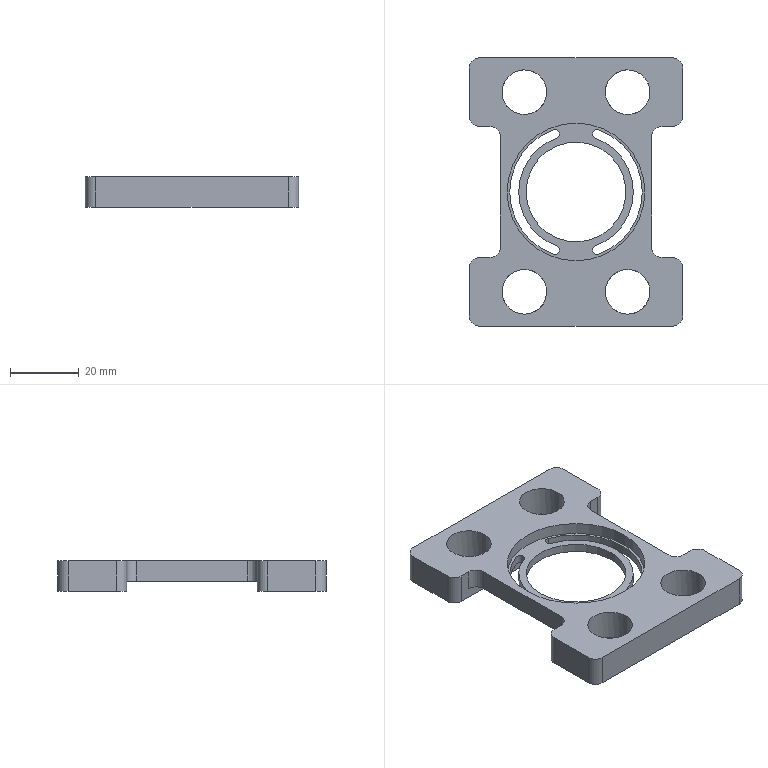Part | 1 solid | 41 faces | box 62 x 78 x 9 mm | volume 20835 mm3 | cylinder 26 | plane 15 | commonest cylinder face diameters 6 x12 2.6 x4 13 x4 33.3 x2 38.5 x2 29 x1
STEP:
#1=CARTESIAN_POINT('',(-25.,-19.,-6.));
#2=VERTEX_POINT('',#1);
#3=CARTESIAN_POINT('',(25.,-19.,-6.));
#4=VERTEX_POINT('',#3);
#5=CARTESIAN_POINT('',(28.,-19.,-6.));
#6=DIRECTION('',(1.,0.,0.));
#7=VECTOR('',#6,1000.);
#8=LINE('',#5,#7);
#9=EDGE_CURVE('',#2,#4,#8,.T.);
#10=ORIENTED_EDGE('',*,*,#9,.F.);
#11=CARTESIAN_POINT('',(-22.,-16.,-6.));
#12=VERTEX_POINT('',#11);
#13=CARTESIAN_POINT('',(-25.,-16.,-6.));
#14=DIRECTION('',(0.,0.,1.));
#15=DIRECTION('',(-1.,0.,0.));
#16=AXIS2_PLACEMENT_3D('',#13,#14,#15);
#17=CIRCLE('',#16,3.);
#18=EDGE_CURVE('',#2,#12,#17,.T.);
#19=ORIENTED_EDGE('',*,*,#18,.T.);
#20=CARTESIAN_POINT('',(-22.,16.,-6.));
#21=VERTEX_POINT('',#20);
#22=CARTESIAN_POINT('',(-22.,-35.,-6.));
#23=DIRECTION('',(0.,1.,0.));
#24=VECTOR('',#23,1000.);
#25=LINE('',#22,#24);
#26=EDGE_CURVE('',#12,#21,#25,.T.);
#27=ORIENTED_EDGE('',*,*,#26,.T.);
#28=CARTESIAN_POINT('',(-25.,19.,-6.));
#29=VERTEX_POINT('',#28);
#30=CARTESIAN_POINT('',(-25.,16.,-6.));
#31=DIRECTION('',(0.,0.,1.));
#32=DIRECTION('',(-1.,0.,0.));
#33=AXIS2_PLACEMENT_3D('',#30,#31,#32);
#34=CIRCLE('',#33,3.);
#35=EDGE_CURVE('',#21,#29,#34,.T.);
#36=ORIENTED_EDGE('',*,*,#35,.T.);
#37=CARTESIAN_POINT('',(25.,19.,-6.));
#38=VERTEX_POINT('',#37);
#39=CARTESIAN_POINT('',(-28.,19.,-6.));
#40=DIRECTION('',(-1.,0.,0.));
#41=VECTOR('',#40,1000.);
#42=LINE('',#39,#41);
#43=EDGE_CURVE('',#38,#29,#42,.T.);
#44=ORIENTED_EDGE('',*,*,#43,.F.);
#45=CARTESIAN_POINT('',(22.,16.,-6.));
#46=VERTEX_POINT('',#45);
#47=CARTESIAN_POINT('',(25.,16.,-6.));
#48=DIRECTION('',(0.,0.,1.));
#49=DIRECTION('',(-1.,0.,0.));
#50=AXIS2_PLACEMENT_3D('',#47,#48,#49);
#51=CIRCLE('',#50,3.);
#52=EDGE_CURVE('',#38,#46,#51,.T.);
#53=ORIENTED_EDGE('',*,*,#52,.T.);
#54=CARTESIAN_POINT('',(22.,-16.,-6.));
#55=VERTEX_POINT('',#54);
#56=CARTESIAN_POINT('',(22.,35.,-6.));
#57=DIRECTION('',(0.,-1.,0.));
#58=VECTOR('',#57,1000.);
#59=LINE('',#56,#58);
#60=EDGE_CURVE('',#46,#55,#59,.T.);
#61=ORIENTED_EDGE('',*,*,#60,.T.);
#62=CARTESIAN_POINT('',(25.,-16.,-6.));
#63=DIRECTION('',(0.,0.,1.));
#64=DIRECTION('',(-1.,0.,0.));
#65=AXIS2_PLACEMENT_3D('',#62,#63,#64);
#66=CIRCLE('',#65,3.);
#67=EDGE_CURVE('',#55,#4,#66,.T.);
#68=ORIENTED_EDGE('',*,*,#67,.T.);
#69=EDGE_LOOP('',(#10,#19,#27,#36,#44,#53,#61,#68));
#70=FACE_BOUND('',#69,.T.);
#71=CARTESIAN_POINT('',(-5.695,-15.646,-6.));
#72=VERTEX_POINT('',#71);
#73=CARTESIAN_POINT('',(-5.695,15.646,-6.));
#74=VERTEX_POINT('',#73);
#75=CARTESIAN_POINT('',(0.,0.,-6.));
#76=DIRECTION('',(0.,0.,-1.));
#77=DIRECTION('',(0.,1.,0.));
#78=AXIS2_PLACEMENT_3D('',#75,#76,#77);
#79=CIRCLE('',#78,16.65);
#80=EDGE_CURVE('',#72,#74,#79,.T.);
#81=ORIENTED_EDGE('',*,*,#80,.T.);
#82=CARTESIAN_POINT('',(-6.584,18.089,-6.));
#83=VERTEX_POINT('',#82);
#84=CARTESIAN_POINT('',(-6.139,16.867,-6.));
#85=DIRECTION('',(0.,0.,1.));
#86=DIRECTION('',(0.,-1.,0.));
#87=AXIS2_PLACEMENT_3D('',#84,#85,#86);
#88=CIRCLE('',#87,1.3);
#89=EDGE_CURVE('',#74,#83,#88,.T.);
#90=ORIENTED_EDGE('',*,*,#89,.T.);
#91=CARTESIAN_POINT('',(-6.584,-18.089,-6.));
#92=VERTEX_POINT('',#91);
#93=CARTESIAN_POINT('',(0.,0.,-6.));
#94=DIRECTION('',(0.,0.,1.));
#95=DIRECTION('',(0.,1.,0.));
#96=AXIS2_PLACEMENT_3D('',#93,#94,#95);
#97=CIRCLE('',#96,19.25);
#98=EDGE_CURVE('',#83,#92,#97,.T.);
#99=ORIENTED_EDGE('',*,*,#98,.T.);
#100=CARTESIAN_POINT('',(-6.139,-16.867,-6.));
#101=DIRECTION('',(0.,0.,1.));
#102=DIRECTION('',(0.,1.,0.));
#103=AXIS2_PLACEMENT_3D('',#100,#101,#102);
#104=CIRCLE('',#103,1.3);
#105=EDGE_CURVE('',#92,#72,#104,.T.);
#106=ORIENTED_EDGE('',*,*,#105,.T.);
#107=EDGE_LOOP('',(#81,#90,#99,#106));
#108=FACE_BOUND('',#107,.T.);
#109=CARTESIAN_POINT('',(6.584,18.089,-6.));
#110=VERTEX_POINT('',#109);
#111=CARTESIAN_POINT('',(5.695,15.646,-6.));
#112=VERTEX_POINT('',#111);
#113=CARTESIAN_POINT('',(6.139,16.867,-6.));
#114=DIRECTION('',(0.,0.,1.));
#115=DIRECTION('',(0.,-1.,0.));
#116=AXIS2_PLACEMENT_3D('',#113,#114,#115);
#117=CIRCLE('',#116,1.3);
#118=EDGE_CURVE('',#110,#112,#117,.T.);
#119=ORIENTED_EDGE('',*,*,#118,.T.);
#120=CARTESIAN_POINT('',(5.695,-15.646,-6.));
#121=VERTEX_POINT('',#120);
#122=CARTESIAN_POINT('',(0.,0.,-6.));
#123=DIRECTION('',(0.,0.,-1.));
#124=DIRECTION('',(0.,1.,0.));
#125=AXIS2_PLACEMENT_3D('',#122,#123,#124);
#126=CIRCLE('',#125,16.65);
#127=EDGE_CURVE('',#112,#121,#126,.T.);
#128=ORIENTED_EDGE('',*,*,#127,.T.);
#129=CARTESIAN_POINT('',(6.584,-18.089,-6.));
#130=VERTEX_POINT('',#129);
#131=CARTESIAN_POINT('',(6.139,-16.867,-6.));
#132=DIRECTION('',(0.,0.,1.));
#133=DIRECTION('',(0.,1.,0.));
#134=AXIS2_PLACEMENT_3D('',#131,#132,#133);
#135=CIRCLE('',#134,1.3);
#136=EDGE_CURVE('',#121,#130,#135,.T.);
#137=ORIENTED_EDGE('',*,*,#136,.T.);
#138=CARTESIAN_POINT('',(0.,0.,-6.));
#139=DIRECTION('',(0.,0.,1.));
#140=DIRECTION('',(0.,1.,0.));
#141=AXIS2_PLACEMENT_3D('',#138,#139,#140);
#142=CIRCLE('',#141,19.25);
#143=EDGE_CURVE('',#130,#110,#142,.T.);
#144=ORIENTED_EDGE('',*,*,#143,.T.);
#145=EDGE_LOOP('',(#119,#128,#137,#144));
#146=FACE_BOUND('',#145,.T.);
#147=CARTESIAN_POINT('',(-14.5,0.,-6.));
#148=VERTEX_POINT('',#147);
#149=CARTESIAN_POINT('',(0.,0.,-6.));
#150=DIRECTION('',(0.,0.,1.));
#151=DIRECTION('',(-1.,0.,0.));
#152=AXIS2_PLACEMENT_3D('',#149,#150,#151);
#153=CIRCLE('',#152,14.5);
#154=EDGE_CURVE('',#148,#148,#153,.T.);
#155=ORIENTED_EDGE('',*,*,#154,.T.);
#156=EDGE_LOOP('',(#155));
#157=FACE_BOUND('',#156,.T.);
#158=CARTESIAN_POINT('',(0.,0.,-6.));
#159=DIRECTION('',(0.,0.,-1.));
#160=DIRECTION('',(1.,0.,0.));
#161=AXIS2_PLACEMENT_3D('',#158,#159,#160);
#162=PLANE('',#161);
#163=ADVANCED_FACE('',(#70,#108,#146,#157),#162,.T.);
#164=CARTESIAN_POINT('',(-5.695,15.646,-3.5));
#165=VERTEX_POINT('',#164);
#166=CARTESIAN_POINT('',(-6.584,18.089,-3.5));
#167=VERTEX_POINT('',#166);
#168=CARTESIAN_POINT('',(-6.139,16.867,-3.5));
#169=DIRECTION('',(0.,0.,1.));
#170=DIRECTION('',(-1.,0.,0.));
#171=AXIS2_PLACEMENT_3D('',#168,#169,#170);
#172=CIRCLE('',#171,1.3);
#173=EDGE_CURVE('',#165,#167,#172,.T.);
#174=ORIENTED_EDGE('',*,*,#173,.F.);
#175=CARTESIAN_POINT('',(-5.695,-15.646,-3.5));
#176=VERTEX_POINT('',#175);
#177=CARTESIAN_POINT('',(0.,0.,-3.5));
#178=DIRECTION('',(0.,0.,-1.));
#179=DIRECTION('',(-1.,0.,0.));
#180=AXIS2_PLACEMENT_3D('',#177,#178,#179);
#181=CIRCLE('',#180,16.65);
#182=EDGE_CURVE('',#176,#165,#181,.T.);
#183=ORIENTED_EDGE('',*,*,#182,.F.);
#184=CARTESIAN_POINT('',(-6.584,-18.089,-3.5));
#185=VERTEX_POINT('',#184);
#186=CARTESIAN_POINT('',(-6.139,-16.867,-3.5));
#187=DIRECTION('',(0.,0.,1.));
#188=DIRECTION('',(-1.,0.,0.));
#189=AXIS2_PLACEMENT_3D('',#186,#187,#188);
#190=CIRCLE('',#189,1.3);
#191=EDGE_CURVE('',#185,#176,#190,.T.);
#192=ORIENTED_EDGE('',*,*,#191,.F.);
#193=CARTESIAN_POINT('',(0.,0.,-3.5));
#194=DIRECTION('',(0.,0.,1.));
#195=DIRECTION('',(-1.,0.,0.));
#196=AXIS2_PLACEMENT_3D('',#193,#194,#195);
#197=CIRCLE('',#196,19.25);
#198=EDGE_CURVE('',#167,#185,#197,.T.);
#199=ORIENTED_EDGE('',*,*,#198,.F.);
#200=EDGE_LOOP('',(#174,#183,#192,#199));
#201=FACE_BOUND('',#200,.T.);
#202=CARTESIAN_POINT('',(5.695,15.646,-3.5));
#203=VERTEX_POINT('',#202);
#204=CARTESIAN_POINT('',(5.695,-15.646,-3.5));
#205=VERTEX_POINT('',#204);
#206=CARTESIAN_POINT('',(0.,0.,-3.5));
#207=DIRECTION('',(0.,0.,-1.));
#208=DIRECTION('',(-1.,0.,0.));
#209=AXIS2_PLACEMENT_3D('',#206,#207,#208);
#210=CIRCLE('',#209,16.65);
#211=EDGE_CURVE('',#203,#205,#210,.T.);
#212=ORIENTED_EDGE('',*,*,#211,.F.);
#213=CARTESIAN_POINT('',(6.584,18.089,-3.5));
#214=VERTEX_POINT('',#213);
#215=CARTESIAN_POINT('',(6.139,16.867,-3.5));
#216=DIRECTION('',(0.,0.,1.));
#217=DIRECTION('',(-1.,0.,0.));
#218=AXIS2_PLACEMENT_3D('',#215,#216,#217);
#219=CIRCLE('',#218,1.3);
#220=EDGE_CURVE('',#214,#203,#219,.T.);
#221=ORIENTED_EDGE('',*,*,#220,.F.);
#222=CARTESIAN_POINT('',(6.584,-18.089,-3.5));
#223=VERTEX_POINT('',#222);
#224=CARTESIAN_POINT('',(0.,0.,-3.5));
#225=DIRECTION('',(0.,0.,1.));
#226=DIRECTION('',(-1.,0.,0.));
#227=AXIS2_PLACEMENT_3D('',#224,#225,#226);
#228=CIRCLE('',#227,19.25);
#229=EDGE_CURVE('',#223,#214,#228,.T.);
#230=ORIENTED_EDGE('',*,*,#229,.F.);
#231=CARTESIAN_POINT('',(6.139,-16.867,-3.5));
#232=DIRECTION('',(0.,0.,1.));
#233=DIRECTION('',(-1.,0.,0.));
#234=AXIS2_PLACEMENT_3D('',#231,#232,#233);
#235=CIRCLE('',#234,1.3);
#236=EDGE_CURVE('',#205,#223,#235,.T.);
#237=ORIENTED_EDGE('',*,*,#236,.F.);
#238=EDGE_LOOP('',(#212,#221,#230,#237));
#239=FACE_BOUND('',#238,.T.);
#240=CARTESIAN_POINT('',(-14.5,0.,-3.5));
#241=VERTEX_POINT('',#240);
#242=CARTESIAN_POINT('',(0.,0.,-3.5));
#243=DIRECTION('',(0.,0.,1.));
#244=DIRECTION('',(-1.,0.,0.));
#245=AXIS2_PLACEMENT_3D('',#242,#243,#244);
#246=CIRCLE('',#245,14.5);
#247=EDGE_CURVE('',#241,#241,#246,.T.);
#248=ORIENTED_EDGE('',*,*,#247,.F.);
#249=EDGE_LOOP('',(#248));
#250=FACE_BOUND('',#249,.T.);
#251=CARTESIAN_POINT('',(-20.,0.,-3.5));
#252=VERTEX_POINT('',#251);
#253=CARTESIAN_POINT('',(0.,0.,-3.5));
#254=DIRECTION('',(0.,0.,1.));
#255=DIRECTION('',(-1.,0.,0.));
#256=AXIS2_PLACEMENT_3D('',#253,#254,#255);
#257=CIRCLE('',#256,20.);
#258=EDGE_CURVE('',#252,#252,#257,.T.);
#259=ORIENTED_EDGE('',*,*,#258,.T.);
#260=EDGE_LOOP('',(#259));
#261=FACE_BOUND('',#260,.T.);
#262=CARTESIAN_POINT('',(0.,0.,-3.5));
#263=DIRECTION('',(0.,0.,-1.));
#264=DIRECTION('',(1.,0.,0.));
#265=AXIS2_PLACEMENT_3D('',#262,#263,#264);
#266=PLANE('',#265);
#267=ADVANCED_FACE('',(#201,#239,#250,#261),#266,.F.);
#268=ORIENTED_EDGE('',*,*,#26,.F.);
#269=CARTESIAN_POINT('',(-22.,-16.,0.));
#270=VERTEX_POINT('',#269);
#271=CARTESIAN_POINT('',(-22.,-16.,-9.));
#272=DIRECTION('',(0.,0.,1.));
#273=VECTOR('',#272,1000.);
#274=LINE('',#271,#273);
#275=EDGE_CURVE('',#12,#270,#274,.T.);
#276=ORIENTED_EDGE('',*,*,#275,.T.);
#277=CARTESIAN_POINT('',(-22.,16.,0.));
#278=VERTEX_POINT('',#277);
#279=CARTESIAN_POINT('',(-22.,-35.,0.));
#280=DIRECTION('',(0.,1.,0.));
#281=VECTOR('',#280,1000.);
#282=LINE('',#279,#281);
#283=EDGE_CURVE('',#270,#278,#282,.T.);
#284=ORIENTED_EDGE('',*,*,#283,.T.);
#285=CARTESIAN_POINT('',(-22.,16.,-9.));
#286=DIRECTION('',(0.,0.,-1.));
#287=VECTOR('',#286,1000.);
#288=LINE('',#285,#287);
#289=EDGE_CURVE('',#278,#21,#288,.T.);
#290=ORIENTED_EDGE('',*,*,#289,.T.);
#291=EDGE_LOOP('',(#268,#276,#284,#290));
#292=FACE_BOUND('',#291,.T.);
#293=CARTESIAN_POINT('',(-22.,-35.,-9.));
#294=DIRECTION('',(1.,0.,0.));
#295=DIRECTION('',(0.,0.,1.));
#296=AXIS2_PLACEMENT_3D('',#293,#294,#295);
#297=PLANE('',#296);
#298=ADVANCED_FACE('',(#292),#297,.F.);
#299=CARTESIAN_POINT('',(-28.,39.,0.));
#300=VERTEX_POINT('',#299);
#301=CARTESIAN_POINT('',(28.,39.,0.));
#302=VERTEX_POINT('',#301);
#303=CARTESIAN_POINT('',(-25.,39.,0.));
#304=DIRECTION('',(1.,0.,0.));
#305=VECTOR('',#304,1000.);
#306=LINE('',#303,#305);
#307=EDGE_CURVE('',#300,#302,#306,.T.);
#308=ORIENTED_EDGE('',*,*,#307,.T.);
#309=CARTESIAN_POINT('',(28.,39.,-9.));
#310=VERTEX_POINT('',#309);
#311=CARTESIAN_POINT('',(28.,39.,-9.));
#312=DIRECTION('',(0.,0.,-1.));
#313=VECTOR('',#312,1000.);
#314=LINE('',#311,#313);
#315=EDGE_CURVE('',#302,#310,#314,.T.);
#316=ORIENTED_EDGE('',*,*,#315,.T.);
#317=CARTESIAN_POINT('',(-28.,39.,-9.));
#318=VERTEX_POINT('',#317);
#319=CARTESIAN_POINT('',(-28.,39.,-9.));
#320=DIRECTION('',(1.,0.,0.));
#321=VECTOR('',#320,1000.);
#322=LINE('',#319,#321);
#323=EDGE_CURVE('',#318,#310,#322,.T.);
#324=ORIENTED_EDGE('',*,*,#323,.F.);
#325=CARTESIAN_POINT('',(-28.,39.,-9.));
#326=DIRECTION('',(0.,0.,1.));
#327=VECTOR('',#326,1000.);
#328=LINE('',#325,#327);
#329=EDGE_CURVE('',#318,#300,#328,.T.);
#330=ORIENTED_EDGE('',*,*,#329,.T.);
#331=EDGE_LOOP('',(#308,#316,#324,#330));
#332=FACE_BOUND('',#331,.T.);
#333=CARTESIAN_POINT('',(-25.,39.,-9.));
#334=DIRECTION('',(0.,-1.,0.));
#335=DIRECTION('',(0.,0.,-1.));
#336=AXIS2_PLACEMENT_3D('',#333,#334,#335);
#337=PLANE('',#336);
#338=ADVANCED_FACE('',(#332),#337,.F.);
#339=CARTESIAN_POINT('',(22.,16.,0.));
#340=VERTEX_POINT('',#339);
#341=CARTESIAN_POINT('',(22.,-16.,0.));
#342=VERTEX_POINT('',#341);
#343=CARTESIAN_POINT('',(22.,35.,0.));
#344=DIRECTION('',(0.,-1.,0.));
#345=VECTOR('',#344,1000.);
#346=LINE('',#343,#345);
#347=EDGE_CURVE('',#340,#342,#346,.T.);
#348=ORIENTED_EDGE('',*,*,#347,.T.);
#349=CARTESIAN_POINT('',(22.,-16.,-9.));
#350=DIRECTION('',(0.,0.,-1.));
#351=VECTOR('',#350,1000.);
#352=LINE('',#349,#351);
#353=EDGE_CURVE('',#342,#55,#352,.T.);
#354=ORIENTED_EDGE('',*,*,#353,.T.);
#355=ORIENTED_EDGE('',*,*,#60,.F.);
#356=CARTESIAN_POINT('',(22.,16.,-9.));
#357=DIRECTION('',(0.,0.,1.));
#358=VECTOR('',#357,1000.);
#359=LINE('',#356,#358);
#360=EDGE_CURVE('',#46,#340,#359,.T.);
#361=ORIENTED_EDGE('',*,*,#360,.T.);
#362=EDGE_LOOP('',(#348,#354,#355,#361));
#363=FACE_BOUND('',#362,.T.);
#364=CARTESIAN_POINT('',(22.,35.,-9.));
#365=DIRECTION('',(-1.,0.,0.));
#366=DIRECTION('',(0.,0.,-1.));
#367=AXIS2_PLACEMENT_3D('',#364,#365,#366);
#368=PLANE('',#367);
#369=ADVANCED_FACE('',(#363),#368,.F.);
#370=ORIENTED_EDGE('',*,*,#258,.F.);
#371=EDGE_LOOP('',(#370));
#372=FACE_BOUND('',#371,.T.);
#373=CARTESIAN_POINT('',(-20.,0.,0.));
#374=VERTEX_POINT('',#373);
#375=CARTESIAN_POINT('',(0.,0.,0.));
#376=DIRECTION('',(0.,0.,1.));
#377=DIRECTION('',(-1.,0.,0.));
#378=AXIS2_PLACEMENT_3D('',#375,#376,#377);
#379=CIRCLE('',#378,20.);
#380=EDGE_CURVE('',#374,#374,#379,.T.);
#381=ORIENTED_EDGE('',*,*,#380,.T.);
#382=EDGE_LOOP('',(#381));
#383=FACE_BOUND('',#382,.T.);
#384=CARTESIAN_POINT('',(0.,0.,-9.));
#385=DIRECTION('',(0.,0.,1.));
#386=DIRECTION('',(-1.,0.,0.));
#387=AXIS2_PLACEMENT_3D('',#384,#385,#386);
#388=CYLINDRICAL_SURFACE('',#387,20.);
#389=ADVANCED_FACE('',(#372,#383),#388,.F.);
#390=CARTESIAN_POINT('',(28.,-39.,0.));
#391=VERTEX_POINT('',#390);
#392=CARTESIAN_POINT('',(-28.,-39.,0.));
#393=VERTEX_POINT('',#392);
#394=CARTESIAN_POINT('',(25.,-39.,0.));
#395=DIRECTION('',(-1.,0.,0.));
#396=VECTOR('',#395,1000.);
#397=LINE('',#394,#396);
#398=EDGE_CURVE('',#391,#393,#397,.T.);
#399=ORIENTED_EDGE('',*,*,#398,.T.);
#400=CARTESIAN_POINT('',(-28.,-39.,-9.));
#401=VERTEX_POINT('',#400);
#402=CARTESIAN_POINT('',(-28.,-39.,-9.));
#403=DIRECTION('',(0.,0.,-1.));
#404=VECTOR('',#403,1000.);
#405=LINE('',#402,#404);
#406=EDGE_CURVE('',#393,#401,#405,.T.);
#407=ORIENTED_EDGE('',*,*,#406,.T.);
#408=CARTESIAN_POINT('',(28.,-39.,-9.));
#409=VERTEX_POINT('',#408);
#410=CARTESIAN_POINT('',(28.,-39.,-9.));
#411=DIRECTION('',(-1.,0.,0.));
#412=VECTOR('',#411,1000.);
#413=LINE('',#410,#412);
#414=EDGE_CURVE('',#409,#401,#413,.T.);
#415=ORIENTED_EDGE('',*,*,#414,.F.);
#416=CARTESIAN_POINT('',(28.,-39.,-9.));
#417=DIRECTION('',(0.,0.,1.));
#418=VECTOR('',#417,1000.);
#419=LINE('',#416,#418);
#420=EDGE_CURVE('',#409,#391,#419,.T.);
#421=ORIENTED_EDGE('',*,*,#420,.T.);
#422=EDGE_LOOP('',(#399,#407,#415,#421));
#423=FACE_BOUND('',#422,.T.);
#424=CARTESIAN_POINT('',(25.,-39.,-9.));
#425=DIRECTION('',(0.,1.,0.));
#426=DIRECTION('',(0.,0.,1.));
#427=AXIS2_PLACEMENT_3D('',#424,#425,#426);
#428=PLANE('',#427);
#429=ADVANCED_FACE('',(#423),#428,.F.);
#430=CARTESIAN_POINT('',(8.5,-29.,0.));
#431=VERTEX_POINT('',#430);
#432=CARTESIAN_POINT('',(15.,-29.,0.));
#433=DIRECTION('',(0.,0.,1.));
#434=DIRECTION('',(-1.,0.,0.));
#435=AXIS2_PLACEMENT_3D('',#432,#433,#434);
#436=CIRCLE('',#435,6.5);
#437=EDGE_CURVE('',#431,#431,#436,.T.);
#438=ORIENTED_EDGE('',*,*,#437,.F.);
#439=EDGE_LOOP('',(#438));
#440=FACE_BOUND('',#439,.T.);
#441=CARTESIAN_POINT('',(-21.5,29.,0.));
#442=VERTEX_POINT('',#441);
#443=CARTESIAN_POINT('',(-15.,29.,0.));
#444=DIRECTION('',(0.,0.,1.));
#445=DIRECTION('',(-1.,0.,0.));
#446=AXIS2_PLACEMENT_3D('',#443,#444,#445);
#447=CIRCLE('',#446,6.5);
#448=EDGE_CURVE('',#442,#442,#447,.T.);
#449=ORIENTED_EDGE('',*,*,#448,.F.);
#450=EDGE_LOOP('',(#449));
#451=FACE_BOUND('',#450,.T.);
#452=CARTESIAN_POINT('',(-21.5,-29.,0.));
#453=VERTEX_POINT('',#452);
#454=CARTESIAN_POINT('',(-15.,-29.,0.));
#455=DIRECTION('',(0.,0.,1.));
#456=DIRECTION('',(-1.,0.,0.));
#457=AXIS2_PLACEMENT_3D('',#454,#455,#456);
#458=CIRCLE('',#457,6.5);
#459=EDGE_CURVE('',#453,#453,#458,.T.);
#460=ORIENTED_EDGE('',*,*,#459,.F.);
#461=EDGE_LOOP('',(#460));
#462=FACE_BOUND('',#461,.T.);
#463=CARTESIAN_POINT('',(8.5,29.,0.));
#464=VERTEX_POINT('',#463);
#465=CARTESIAN_POINT('',(15.,29.,0.));
#466=DIRECTION('',(0.,0.,1.));
#467=DIRECTION('',(-1.,0.,0.));
#468=AXIS2_PLACEMENT_3D('',#465,#466,#467);
#469=CIRCLE('',#468,6.5);
#470=EDGE_CURVE('',#464,#464,#469,.T.);
#471=ORIENTED_EDGE('',*,*,#470,.F.);
#472=EDGE_LOOP('',(#471));
#473=FACE_BOUND('',#472,.T.);
#474=ORIENTED_EDGE('',*,*,#380,.F.);
#475=EDGE_LOOP('',(#474));
#476=FACE_BOUND('',#475,.T.);
#477=CARTESIAN_POINT('',(25.,19.,0.));
#478=VERTEX_POINT('',#477);
#479=CARTESIAN_POINT('',(28.,19.,0.));
#480=VERTEX_POINT('',#479);
#481=CARTESIAN_POINT('',(31.,19.,0.));
#482=DIRECTION('',(-1.,0.,0.));
#483=VECTOR('',#482,1000.);
#484=LINE('',#481,#483);
#485=EDGE_CURVE('',#478,#480,#484,.F.);
#486=ORIENTED_EDGE('',*,*,#485,.T.);
#487=CARTESIAN_POINT('',(31.,22.,0.));
#488=VERTEX_POINT('',#487);
#489=CARTESIAN_POINT('',(28.,22.,0.));
#490=DIRECTION('',(0.,0.,1.));
#491=DIRECTION('',(-1.,0.,0.));
#492=AXIS2_PLACEMENT_3D('',#489,#490,#491);
#493=CIRCLE('',#492,3.);
#494=EDGE_CURVE('',#480,#488,#493,.T.);
#495=ORIENTED_EDGE('',*,*,#494,.T.);
#496=CARTESIAN_POINT('',(31.,36.,0.));
#497=VERTEX_POINT('',#496);
#498=CARTESIAN_POINT('',(31.,39.,0.));
#499=DIRECTION('',(0.,1.,0.));
#500=VECTOR('',#499,1000.);
#501=LINE('',#498,#500);
#502=EDGE_CURVE('',#488,#497,#501,.T.);
#503=ORIENTED_EDGE('',*,*,#502,.T.);
#504=CARTESIAN_POINT('',(28.,36.,0.));
#505=DIRECTION('',(0.,0.,1.));
#506=DIRECTION('',(-1.,0.,0.));
#507=AXIS2_PLACEMENT_3D('',#504,#505,#506);
#508=CIRCLE('',#507,3.);
#509=EDGE_CURVE('',#497,#302,#508,.T.);
#510=ORIENTED_EDGE('',*,*,#509,.T.);
#511=ORIENTED_EDGE('',*,*,#307,.F.);
#512=CARTESIAN_POINT('',(-31.,36.,0.));
#513=VERTEX_POINT('',#512);
#514=CARTESIAN_POINT('',(-28.,36.,0.));
#515=DIRECTION('',(0.,0.,1.));
#516=DIRECTION('',(-1.,0.,0.));
#517=AXIS2_PLACEMENT_3D('',#514,#515,#516);
#518=CIRCLE('',#517,3.);
#519=EDGE_CURVE('',#300,#513,#518,.T.);
#520=ORIENTED_EDGE('',*,*,#519,.T.);
#521=CARTESIAN_POINT('',(-31.,22.,0.));
#522=VERTEX_POINT('',#521);
#523=CARTESIAN_POINT('',(-31.,19.,0.));
#524=DIRECTION('',(0.,-1.,0.));
#525=VECTOR('',#524,1000.);
#526=LINE('',#523,#525);
#527=EDGE_CURVE('',#513,#522,#526,.T.);
#528=ORIENTED_EDGE('',*,*,#527,.T.);
#529=CARTESIAN_POINT('',(-28.,19.,0.));
#530=VERTEX_POINT('',#529);
#531=CARTESIAN_POINT('',(-28.,22.,0.));
#532=DIRECTION('',(0.,0.,1.));
#533=DIRECTION('',(-1.,0.,0.));
#534=AXIS2_PLACEMENT_3D('',#531,#532,#533);
#535=CIRCLE('',#534,3.);
#536=EDGE_CURVE('',#522,#530,#535,.T.);
#537=ORIENTED_EDGE('',*,*,#536,.T.);
#538=CARTESIAN_POINT('',(-25.,19.,0.));
#539=VERTEX_POINT('',#538);
#540=CARTESIAN_POINT('',(-30.,19.,0.));
#541=DIRECTION('',(1.,0.,0.));
#542=VECTOR('',#541,1000.);
#543=LINE('',#540,#542);
#544=EDGE_CURVE('',#539,#530,#543,.F.);
#545=ORIENTED_EDGE('',*,*,#544,.F.);
#546=CARTESIAN_POINT('',(-25.,16.,0.));
#547=DIRECTION('',(0.,0.,-1.));
#548=DIRECTION('',(-1.,0.,0.));
#549=AXIS2_PLACEMENT_3D('',#546,#547,#548);
#550=CIRCLE('',#549,3.);
#551=EDGE_CURVE('',#539,#278,#550,.T.);
#552=ORIENTED_EDGE('',*,*,#551,.T.);
#553=ORIENTED_EDGE('',*,*,#283,.F.);
#554=CARTESIAN_POINT('',(-25.,-19.,0.));
#555=VERTEX_POINT('',#554);
#556=CARTESIAN_POINT('',(-25.,-16.,0.));
#557=DIRECTION('',(0.,0.,-1.));
#558=DIRECTION('',(-1.,0.,0.));
#559=AXIS2_PLACEMENT_3D('',#556,#557,#558);
#560=CIRCLE('',#559,3.);
#561=EDGE_CURVE('',#270,#555,#560,.T.);
#562=ORIENTED_EDGE('',*,*,#561,.T.);
#563=CARTESIAN_POINT('',(-28.,-19.,0.));
#564=VERTEX_POINT('',#563);
#565=CARTESIAN_POINT('',(-30.,-19.,0.));
#566=DIRECTION('',(1.,0.,0.));
#567=VECTOR('',#566,1000.);
#568=LINE('',#565,#567);
#569=EDGE_CURVE('',#555,#564,#568,.F.);
#570=ORIENTED_EDGE('',*,*,#569,.T.);
#571=CARTESIAN_POINT('',(-31.,-22.,0.));
#572=VERTEX_POINT('',#571);
#573=CARTESIAN_POINT('',(-28.,-22.,0.));
#574=DIRECTION('',(0.,0.,1.));
#575=DIRECTION('',(-1.,0.,0.));
#576=AXIS2_PLACEMENT_3D('',#573,#574,#575);
#577=CIRCLE('',#576,3.);
#578=EDGE_CURVE('',#564,#572,#577,.T.);
#579=ORIENTED_EDGE('',*,*,#578,.T.);
#580=CARTESIAN_POINT('',(-31.,-36.,0.));
#581=VERTEX_POINT('',#580);
#582=CARTESIAN_POINT('',(-31.,-39.,0.));
#583=DIRECTION('',(0.,-1.,0.));
#584=VECTOR('',#583,1000.);
#585=LINE('',#582,#584);
#586=EDGE_CURVE('',#572,#581,#585,.T.);
#587=ORIENTED_EDGE('',*,*,#586,.T.);
#588=CARTESIAN_POINT('',(-28.,-36.,0.));
#589=DIRECTION('',(0.,0.,1.));
#590=DIRECTION('',(-1.,0.,0.));
#591=AXIS2_PLACEMENT_3D('',#588,#589,#590);
#592=CIRCLE('',#591,3.);
#593=EDGE_CURVE('',#581,#393,#592,.T.);
#594=ORIENTED_EDGE('',*,*,#593,.T.);
#595=ORIENTED_EDGE('',*,*,#398,.F.);
#596=CARTESIAN_POINT('',(31.,-36.,0.));
#597=VERTEX_POINT('',#596);
#598=CARTESIAN_POINT('',(28.,-36.,0.));
#599=DIRECTION('',(0.,0.,1.));
#600=DIRECTION('',(-1.,0.,0.));
#601=AXIS2_PLACEMENT_3D('',#598,#599,#600);
#602=CIRCLE('',#601,3.);
#603=EDGE_CURVE('',#391,#597,#602,.T.);
#604=ORIENTED_EDGE('',*,*,#603,.T.);
#605=CARTESIAN_POINT('',(31.,-22.,0.));
#606=VERTEX_POINT('',#605);
#607=CARTESIAN_POINT('',(31.,-19.,0.));
#608=DIRECTION('',(0.,1.,0.));
#609=VECTOR('',#608,1000.);
#610=LINE('',#607,#609);
#611=EDGE_CURVE('',#597,#606,#610,.T.);
#612=ORIENTED_EDGE('',*,*,#611,.T.);
#613=CARTESIAN_POINT('',(28.,-19.,0.));
#614=VERTEX_POINT('',#613);
#615=CARTESIAN_POINT('',(28.,-22.,0.));
#616=DIRECTION('',(0.,0.,1.));
#617=DIRECTION('',(-1.,0.,0.));
#618=AXIS2_PLACEMENT_3D('',#615,#616,#617);
#619=CIRCLE('',#618,3.);
#620=EDGE_CURVE('',#606,#614,#619,.T.);
#621=ORIENTED_EDGE('',*,*,#620,.T.);
#622=CARTESIAN_POINT('',(25.,-19.,0.));
#623=VERTEX_POINT('',#622);
#624=CARTESIAN_POINT('',(31.,-19.,0.));
#625=DIRECTION('',(-1.,0.,0.));
#626=VECTOR('',#625,1000.);
#627=LINE('',#624,#626);
#628=EDGE_CURVE('',#623,#614,#627,.F.);
#629=ORIENTED_EDGE('',*,*,#628,.F.);
#630=CARTESIAN_POINT('',(25.,-16.,0.));
#631=DIRECTION('',(0.,0.,-1.));
#632=DIRECTION('',(-1.,0.,0.));
#633=AXIS2_PLACEMENT_3D('',#630,#631,#632);
#634=CIRCLE('',#633,3.);
#635=EDGE_CURVE('',#623,#342,#634,.T.);
#636=ORIENTED_EDGE('',*,*,#635,.T.);
#637=ORIENTED_EDGE('',*,*,#347,.F.);
#638=CARTESIAN_POINT('',(25.,16.,0.));
#639=DIRECTION('',(0.,0.,-1.));
#640=DIRECTION('',(-1.,0.,0.));
#641=AXIS2_PLACEMENT_3D('',#638,#639,#640);
#642=CIRCLE('',#641,3.);
#643=EDGE_CURVE('',#340,#478,#642,.T.);
#644=ORIENTED_EDGE('',*,*,#643,.T.);
#645=EDGE_LOOP('',(#486,#495,#503,#510,#511,#520,#528,#537,#545,#552,#553,#562,#570,#579,#587,#594,#595,#604,#612,#621,#629,#636,#637,#644));
#646=FACE_BOUND('',#645,.T.);
#647=CARTESIAN_POINT('',(0.,0.,0.));
#648=DIRECTION('',(0.,0.,-1.));
#649=DIRECTION('',(1.,0.,0.));
#650=AXIS2_PLACEMENT_3D('',#647,#648,#649);
#651=PLANE('',#650);
#652=ADVANCED_FACE('',(#440,#451,#462,#473,#476,#646),#651,.F.);
#653=ORIENTED_EDGE('',*,*,#154,.F.);
#654=EDGE_LOOP('',(#653));
#655=FACE_BOUND('',#654,.T.);
#656=ORIENTED_EDGE('',*,*,#247,.T.);
#657=EDGE_LOOP('',(#656));
#658=FACE_BOUND('',#657,.T.);
#659=CARTESIAN_POINT('',(0.,0.,-6.));
#660=DIRECTION('',(0.,0.,1.));
#661=DIRECTION('',(-1.,0.,0.));
#662=AXIS2_PLACEMENT_3D('',#659,#660,#661);
#663=CYLINDRICAL_SURFACE('',#662,14.5);
#664=ADVANCED_FACE('',(#655,#658),#663,.F.);
#665=ORIENTED_EDGE('',*,*,#211,.T.);
#666=CARTESIAN_POINT('',(5.695,-15.646,5.087));
#667=DIRECTION('',(0.,0.,-1.));
#668=VECTOR('',#667,1000.);
#669=LINE('',#666,#668);
#670=EDGE_CURVE('',#205,#121,#669,.T.);
#671=ORIENTED_EDGE('',*,*,#670,.T.);
#672=ORIENTED_EDGE('',*,*,#127,.F.);
#673=CARTESIAN_POINT('',(5.695,15.646,5.087));
#674=DIRECTION('',(0.,0.,-1.));
#675=VECTOR('',#674,1000.);
#676=LINE('',#673,#675);
#677=EDGE_CURVE('',#203,#112,#676,.T.);
#678=ORIENTED_EDGE('',*,*,#677,.F.);
#679=EDGE_LOOP('',(#665,#671,#672,#678));
#680=FACE_BOUND('',#679,.T.);
#681=CARTESIAN_POINT('',(0.,0.,5.087));
#682=DIRECTION('',(0.,0.,-1.));
#683=DIRECTION('',(1.,0.,0.));
#684=AXIS2_PLACEMENT_3D('',#681,#682,#683);
#685=CYLINDRICAL_SURFACE('',#684,16.65);
#686=ADVANCED_FACE('',(#680),#685,.T.);
#687=ORIENTED_EDGE('',*,*,#236,.T.);
#688=CARTESIAN_POINT('',(6.584,-18.089,5.087));
#689=DIRECTION('',(0.,0.,-1.));
#690=VECTOR('',#689,1000.);
#691=LINE('',#688,#690);
#692=EDGE_CURVE('',#223,#130,#691,.T.);
#693=ORIENTED_EDGE('',*,*,#692,.T.);
#694=ORIENTED_EDGE('',*,*,#136,.F.);
#695=ORIENTED_EDGE('',*,*,#670,.F.);
#696=EDGE_LOOP('',(#687,#693,#694,#695));
#697=FACE_BOUND('',#696,.T.);
#698=CARTESIAN_POINT('',(6.139,-16.867,5.087));
#699=DIRECTION('',(0.,0.,-1.));
#700=DIRECTION('',(1.,0.,0.));
#701=AXIS2_PLACEMENT_3D('',#698,#699,#700);
#702=CYLINDRICAL_SURFACE('',#701,1.3);
#703=ADVANCED_FACE('',(#697),#702,.F.);
#704=ORIENTED_EDGE('',*,*,#229,.T.);
#705=CARTESIAN_POINT('',(6.584,18.089,5.087));
#706=DIRECTION('',(0.,0.,-1.));
#707=VECTOR('',#706,1000.);
#708=LINE('',#705,#707);
#709=EDGE_CURVE('',#214,#110,#708,.T.);
#710=ORIENTED_EDGE('',*,*,#709,.T.);
#711=ORIENTED_EDGE('',*,*,#143,.F.);
#712=ORIENTED_EDGE('',*,*,#692,.F.);
#713=EDGE_LOOP('',(#704,#710,#711,#712));
#714=FACE_BOUND('',#713,.T.);
#715=CARTESIAN_POINT('',(0.,0.,5.087));
#716=DIRECTION('',(0.,0.,-1.));
#717=DIRECTION('',(1.,0.,0.));
#718=AXIS2_PLACEMENT_3D('',#715,#716,#717);
#719=CYLINDRICAL_SURFACE('',#718,19.25);
#720=ADVANCED_FACE('',(#714),#719,.F.);
#721=ORIENTED_EDGE('',*,*,#220,.T.);
#722=ORIENTED_EDGE('',*,*,#677,.T.);
#723=ORIENTED_EDGE('',*,*,#118,.F.);
#724=ORIENTED_EDGE('',*,*,#709,.F.);
#725=EDGE_LOOP('',(#721,#722,#723,#724));
#726=FACE_BOUND('',#725,.T.);
#727=CARTESIAN_POINT('',(6.139,16.867,5.087));
#728=DIRECTION('',(0.,0.,-1.));
#729=DIRECTION('',(1.,0.,0.));
#730=AXIS2_PLACEMENT_3D('',#727,#728,#729);
#731=CYLINDRICAL_SURFACE('',#730,1.3);
#732=ADVANCED_FACE('',(#726),#731,.F.);
#733=ORIENTED_EDGE('',*,*,#173,.T.);
#734=CARTESIAN_POINT('',(-6.584,18.089,5.087));
#735=DIRECTION('',(0.,0.,-1.));
#736=VECTOR('',#735,1000.);
#737=LINE('',#734,#736);
#738=EDGE_CURVE('',#167,#83,#737,.T.);
#739=ORIENTED_EDGE('',*,*,#738,.T.);
#740=ORIENTED_EDGE('',*,*,#89,.F.);
#741=CARTESIAN_POINT('',(-5.695,15.646,5.087));
#742=DIRECTION('',(0.,0.,-1.));
#743=VECTOR('',#742,1000.);
#744=LINE('',#741,#743);
#745=EDGE_CURVE('',#165,#74,#744,.T.);
#746=ORIENTED_EDGE('',*,*,#745,.F.);
#747=EDGE_LOOP('',(#733,#739,#740,#746));
#748=FACE_BOUND('',#747,.T.);
#749=CARTESIAN_POINT('',(-6.139,16.867,5.087));
#750=DIRECTION('',(0.,0.,-1.));
#751=DIRECTION('',(1.,0.,0.));
#752=AXIS2_PLACEMENT_3D('',#749,#750,#751);
#753=CYLINDRICAL_SURFACE('',#752,1.3);
#754=ADVANCED_FACE('',(#748),#753,.F.);
#755=ORIENTED_EDGE('',*,*,#198,.T.);
#756=CARTESIAN_POINT('',(-6.584,-18.089,5.087));
#757=DIRECTION('',(0.,0.,-1.));
#758=VECTOR('',#757,1000.);
#759=LINE('',#756,#758);
#760=EDGE_CURVE('',#185,#92,#759,.T.);
#761=ORIENTED_EDGE('',*,*,#760,.T.);
#762=ORIENTED_EDGE('',*,*,#98,.F.);
#763=ORIENTED_EDGE('',*,*,#738,.F.);
#764=EDGE_LOOP('',(#755,#761,#762,#763));
#765=FACE_BOUND('',#764,.T.);
#766=CARTESIAN_POINT('',(0.,0.,5.087));
#767=DIRECTION('',(0.,0.,-1.));
#768=DIRECTION('',(1.,0.,0.));
#769=AXIS2_PLACEMENT_3D('',#766,#767,#768);
#770=CYLINDRICAL_SURFACE('',#769,19.25);
#771=ADVANCED_FACE('',(#765),#770,.F.);
#772=ORIENTED_EDGE('',*,*,#191,.T.);
#773=CARTESIAN_POINT('',(-5.695,-15.646,5.087));
#774=DIRECTION('',(0.,0.,-1.));
#775=VECTOR('',#774,1000.);
#776=LINE('',#773,#775);
#777=EDGE_CURVE('',#176,#72,#776,.T.);
#778=ORIENTED_EDGE('',*,*,#777,.T.);
#779=ORIENTED_EDGE('',*,*,#105,.F.);
#780=ORIENTED_EDGE('',*,*,#760,.F.);
#781=EDGE_LOOP('',(#772,#778,#779,#780));
#782=FACE_BOUND('',#781,.T.);
#783=CARTESIAN_POINT('',(-6.139,-16.867,5.087));
#784=DIRECTION('',(0.,0.,-1.));
#785=DIRECTION('',(1.,0.,0.));
#786=AXIS2_PLACEMENT_3D('',#783,#784,#785);
#787=CYLINDRICAL_SURFACE('',#786,1.3);
#788=ADVANCED_FACE('',(#782),#787,.F.);
#789=ORIENTED_EDGE('',*,*,#182,.T.);
#790=ORIENTED_EDGE('',*,*,#745,.T.);
#791=ORIENTED_EDGE('',*,*,#80,.F.);
#792=ORIENTED_EDGE('',*,*,#777,.F.);
#793=EDGE_LOOP('',(#789,#790,#791,#792));
#794=FACE_BOUND('',#793,.T.);
#795=CARTESIAN_POINT('',(0.,0.,5.087));
#796=DIRECTION('',(0.,0.,-1.));
#797=DIRECTION('',(1.,0.,0.));
#798=AXIS2_PLACEMENT_3D('',#795,#796,#797);
#799=CYLINDRICAL_SURFACE('',#798,16.65);
#800=ADVANCED_FACE('',(#794),#799,.T.);
#801=ORIENTED_EDGE('',*,*,#470,.T.);
#802=EDGE_LOOP('',(#801));
#803=FACE_BOUND('',#802,.T.);
#804=CARTESIAN_POINT('',(15.,22.5,-9.));
#805=VERTEX_POINT('',#804);
#806=CARTESIAN_POINT('',(15.,29.,-9.));
#807=DIRECTION('',(0.,0.,1.));
#808=DIRECTION('',(0.,-1.,0.));
#809=AXIS2_PLACEMENT_3D('',#806,#807,#808);
#810=CIRCLE('',#809,6.5);
#811=EDGE_CURVE('',#805,#805,#810,.T.);
#812=ORIENTED_EDGE('',*,*,#811,.F.);
#813=EDGE_LOOP('',(#812));
#814=FACE_BOUND('',#813,.T.);
#815=CARTESIAN_POINT('',(15.,29.,31.724));
#816=DIRECTION('',(0.,0.,-1.));
#817=DIRECTION('',(1.,0.,0.));
#818=AXIS2_PLACEMENT_3D('',#815,#816,#817);
#819=CYLINDRICAL_SURFACE('',#818,6.5);
#820=ADVANCED_FACE('',(#803,#814),#819,.F.);
#821=ORIENTED_EDGE('',*,*,#437,.T.);
#822=EDGE_LOOP('',(#821));
#823=FACE_BOUND('',#822,.T.);
#824=CARTESIAN_POINT('',(15.,-35.5,-9.));
#825=VERTEX_POINT('',#824);
#826=CARTESIAN_POINT('',(15.,-29.,-9.));
#827=DIRECTION('',(0.,0.,1.));
#828=DIRECTION('',(0.,-1.,0.));
#829=AXIS2_PLACEMENT_3D('',#826,#827,#828);
#830=CIRCLE('',#829,6.5);
#831=EDGE_CURVE('',#825,#825,#830,.T.);
#832=ORIENTED_EDGE('',*,*,#831,.F.);
#833=EDGE_LOOP('',(#832));
#834=FACE_BOUND('',#833,.T.);
#835=CARTESIAN_POINT('',(15.,-29.,31.724));
#836=DIRECTION('',(0.,0.,-1.));
#837=DIRECTION('',(1.,0.,0.));
#838=AXIS2_PLACEMENT_3D('',#835,#836,#837);
#839=CYLINDRICAL_SURFACE('',#838,6.5);
#840=ADVANCED_FACE('',(#823,#834),#839,.F.);
#841=ORIENTED_EDGE('',*,*,#459,.T.);
#842=EDGE_LOOP('',(#841));
#843=FACE_BOUND('',#842,.T.);
#844=CARTESIAN_POINT('',(-15.,-35.5,-9.));
#845=VERTEX_POINT('',#844);
#846=CARTESIAN_POINT('',(-15.,-29.,-9.));
#847=DIRECTION('',(0.,0.,1.));
#848=DIRECTION('',(0.,-1.,0.));
#849=AXIS2_PLACEMENT_3D('',#846,#847,#848);
#850=CIRCLE('',#849,6.5);
#851=EDGE_CURVE('',#845,#845,#850,.T.);
#852=ORIENTED_EDGE('',*,*,#851,.F.);
#853=EDGE_LOOP('',(#852));
#854=FACE_BOUND('',#853,.T.);
#855=CARTESIAN_POINT('',(-15.,-29.,31.724));
#856=DIRECTION('',(0.,0.,-1.));
#857=DIRECTION('',(1.,0.,0.));
#858=AXIS2_PLACEMENT_3D('',#855,#856,#857);
#859=CYLINDRICAL_SURFACE('',#858,6.5);
#860=ADVANCED_FACE('',(#843,#854),#859,.F.);
#861=ORIENTED_EDGE('',*,*,#448,.T.);
#862=EDGE_LOOP('',(#861));
#863=FACE_BOUND('',#862,.T.);
#864=CARTESIAN_POINT('',(-15.,22.5,-9.));
#865=VERTEX_POINT('',#864);
#866=CARTESIAN_POINT('',(-15.,29.,-9.));
#867=DIRECTION('',(0.,0.,1.));
#868=DIRECTION('',(0.,-1.,0.));
#869=AXIS2_PLACEMENT_3D('',#866,#867,#868);
#870=CIRCLE('',#869,6.5);
#871=EDGE_CURVE('',#865,#865,#870,.T.);
#872=ORIENTED_EDGE('',*,*,#871,.F.);
#873=EDGE_LOOP('',(#872));
#874=FACE_BOUND('',#873,.T.);
#875=CARTESIAN_POINT('',(-15.,29.,31.724));
#876=DIRECTION('',(0.,0.,-1.));
#877=DIRECTION('',(1.,0.,0.));
#878=AXIS2_PLACEMENT_3D('',#875,#876,#877);
#879=CYLINDRICAL_SURFACE('',#878,6.5);
#880=ADVANCED_FACE('',(#863,#874),#879,.F.);
#881=ORIENTED_EDGE('',*,*,#527,.F.);
#882=CARTESIAN_POINT('',(-31.,36.,-9.));
#883=VERTEX_POINT('',#882);
#884=CARTESIAN_POINT('',(-31.,36.,0.));
#885=DIRECTION('',(0.,0.,-1.));
#886=VECTOR('',#885,1000.);
#887=LINE('',#884,#886);
#888=EDGE_CURVE('',#513,#883,#887,.T.);
#889=ORIENTED_EDGE('',*,*,#888,.T.);
#890=CARTESIAN_POINT('',(-31.,22.,-9.));
#891=VERTEX_POINT('',#890);
#892=CARTESIAN_POINT('',(-31.,22.,-9.));
#893=DIRECTION('',(0.,1.,0.));
#894=VECTOR('',#893,1000.);
#895=LINE('',#892,#894);
#896=EDGE_CURVE('',#891,#883,#895,.T.);
#897=ORIENTED_EDGE('',*,*,#896,.F.);
#898=CARTESIAN_POINT('',(-31.,22.,0.));
#899=DIRECTION('',(0.,0.,1.));
#900=VECTOR('',#899,1000.);
#901=LINE('',#898,#900);
#902=EDGE_CURVE('',#891,#522,#901,.T.);
#903=ORIENTED_EDGE('',*,*,#902,.T.);
#904=EDGE_LOOP('',(#881,#889,#897,#903));
#905=FACE_BOUND('',#904,.T.);
#906=CARTESIAN_POINT('',(-31.,0.,0.));
#907=DIRECTION('',(1.,0.,0.));
#908=DIRECTION('',(0.,0.,1.));
#909=AXIS2_PLACEMENT_3D('',#906,#907,#908);
#910=PLANE('',#909);
#911=ADVANCED_FACE('',(#905),#910,.F.);
#912=ORIENTED_EDGE('',*,*,#544,.T.);
#913=CARTESIAN_POINT('',(-28.,19.,-9.));
#914=VERTEX_POINT('',#913);
#915=CARTESIAN_POINT('',(-28.,19.,-6.));
#916=DIRECTION('',(0.,0.,-1.));
#917=VECTOR('',#916,1000.);
#918=LINE('',#915,#917);
#919=EDGE_CURVE('',#530,#914,#918,.T.);
#920=ORIENTED_EDGE('',*,*,#919,.T.);
#921=CARTESIAN_POINT('',(28.,19.,-9.));
#922=VERTEX_POINT('',#921);
#923=CARTESIAN_POINT('',(-28.,19.,-9.));
#924=DIRECTION('',(-1.,0.,0.));
#925=VECTOR('',#924,1000.);
#926=LINE('',#923,#925);
#927=EDGE_CURVE('',#922,#914,#926,.T.);
#928=ORIENTED_EDGE('',*,*,#927,.F.);
#929=CARTESIAN_POINT('',(28.,19.,0.));
#930=DIRECTION('',(0.,0.,1.));
#931=VECTOR('',#930,1000.);
#932=LINE('',#929,#931);
#933=EDGE_CURVE('',#922,#480,#932,.T.);
#934=ORIENTED_EDGE('',*,*,#933,.T.);
#935=ORIENTED_EDGE('',*,*,#485,.F.);
#936=CARTESIAN_POINT('',(25.,19.,-6.));
#937=DIRECTION('',(0.,0.,-1.));
#938=VECTOR('',#937,1000.);
#939=LINE('',#936,#938);
#940=EDGE_CURVE('',#478,#38,#939,.T.);
#941=ORIENTED_EDGE('',*,*,#940,.T.);
#942=ORIENTED_EDGE('',*,*,#43,.T.);
#943=CARTESIAN_POINT('',(-25.,19.,-6.));
#944=DIRECTION('',(0.,0.,1.));
#945=VECTOR('',#944,1000.);
#946=LINE('',#943,#945);
#947=EDGE_CURVE('',#29,#539,#946,.T.);
#948=ORIENTED_EDGE('',*,*,#947,.T.);
#949=EDGE_LOOP('',(#912,#920,#928,#934,#935,#941,#942,#948));
#950=FACE_BOUND('',#949,.T.);
#951=CARTESIAN_POINT('',(-30.,19.,-6.));
#952=DIRECTION('',(0.,-1.,0.));
#953=DIRECTION('',(0.,0.,-1.));
#954=AXIS2_PLACEMENT_3D('',#951,#952,#953);
#955=PLANE('',#954);
#956=ADVANCED_FACE('',(#950),#955,.T.);
#957=ORIENTED_EDGE('',*,*,#586,.F.);
#958=CARTESIAN_POINT('',(-31.,-22.,-9.));
#959=VERTEX_POINT('',#958);
#960=CARTESIAN_POINT('',(-31.,-22.,-6.));
#961=DIRECTION('',(0.,0.,-1.));
#962=VECTOR('',#961,1000.);
#963=LINE('',#960,#962);
#964=EDGE_CURVE('',#572,#959,#963,.T.);
#965=ORIENTED_EDGE('',*,*,#964,.T.);
#966=CARTESIAN_POINT('',(-31.,-36.,-9.));
#967=VERTEX_POINT('',#966);
#968=CARTESIAN_POINT('',(-31.,-36.,-9.));
#969=DIRECTION('',(0.,1.,0.));
#970=VECTOR('',#969,1000.);
#971=LINE('',#968,#970);
#972=EDGE_CURVE('',#967,#959,#971,.T.);
#973=ORIENTED_EDGE('',*,*,#972,.F.);
#974=CARTESIAN_POINT('',(-31.,-36.,0.));
#975=DIRECTION('',(0.,0.,1.));
#976=VECTOR('',#975,1000.);
#977=LINE('',#974,#976);
#978=EDGE_CURVE('',#967,#581,#977,.T.);
#979=ORIENTED_EDGE('',*,*,#978,.T.);
#980=EDGE_LOOP('',(#957,#965,#973,#979));
#981=FACE_BOUND('',#980,.T.);
#982=CARTESIAN_POINT('',(-31.,0.,0.));
#983=DIRECTION('',(1.,0.,0.));
#984=DIRECTION('',(0.,0.,1.));
#985=AXIS2_PLACEMENT_3D('',#982,#983,#984);
#986=PLANE('',#985);
#987=ADVANCED_FACE('',(#981),#986,.F.);
#988=CARTESIAN_POINT('',(-25.,-19.,-6.));
#989=DIRECTION('',(0.,0.,-1.));
#990=VECTOR('',#989,1000.);
#991=LINE('',#988,#990);
#992=EDGE_CURVE('',#555,#2,#991,.T.);
#993=ORIENTED_EDGE('',*,*,#992,.T.);
#994=ORIENTED_EDGE('',*,*,#9,.T.);
#995=CARTESIAN_POINT('',(25.,-19.,-6.));
#996=DIRECTION('',(0.,0.,1.));
#997=VECTOR('',#996,1000.);
#998=LINE('',#995,#997);
#999=EDGE_CURVE('',#4,#623,#998,.T.);
#1000=ORIENTED_EDGE('',*,*,#999,.T.);
#1001=ORIENTED_EDGE('',*,*,#628,.T.);
#1002=CARTESIAN_POINT('',(28.,-19.,-9.));
#1003=VERTEX_POINT('',#1002);
#1004=CARTESIAN_POINT('',(28.,-19.,-6.));
#1005=DIRECTION('',(0.,0.,-1.));
#1006=VECTOR('',#1005,1000.);
#1007=LINE('',#1004,#1006);
#1008=EDGE_CURVE('',#614,#1003,#1007,.T.);
#1009=ORIENTED_EDGE('',*,*,#1008,.T.);
#1010=CARTESIAN_POINT('',(-28.,-19.,-9.));
#1011=VERTEX_POINT('',#1010);
#1012=CARTESIAN_POINT('',(-28.,-19.,-9.));
#1013=DIRECTION('',(1.,0.,0.));
#1014=VECTOR('',#1013,1000.);
#1015=LINE('',#1012,#1014);
#1016=EDGE_CURVE('',#1011,#1003,#1015,.T.);
#1017=ORIENTED_EDGE('',*,*,#1016,.F.);
#1018=CARTESIAN_POINT('',(-28.,-19.,0.));
#1019=DIRECTION('',(0.,0.,1.));
#1020=VECTOR('',#1019,1000.);
#1021=LINE('',#1018,#1020);
#1022=EDGE_CURVE('',#1011,#564,#1021,.T.);
#1023=ORIENTED_EDGE('',*,*,#1022,.T.);
#1024=ORIENTED_EDGE('',*,*,#569,.F.);
#1025=EDGE_LOOP('',(#993,#994,#1000,#1001,#1009,#1017,#1023,#1024));
#1026=FACE_BOUND('',#1025,.T.);
#1027=CARTESIAN_POINT('',(-30.,-19.,-6.));
#1028=DIRECTION('',(0.,1.,0.));
#1029=DIRECTION('',(0.,0.,1.));
#1030=AXIS2_PLACEMENT_3D('',#1027,#1028,#1029);
#1031=PLANE('',#1030);
#1032=ADVANCED_FACE('',(#1026),#1031,.T.);
#1033=ORIENTED_EDGE('',*,*,#502,.F.);
#1034=CARTESIAN_POINT('',(31.,22.,-9.));
#1035=VERTEX_POINT('',#1034);
#1036=CARTESIAN_POINT('',(31.,22.,-6.));
#1037=DIRECTION('',(0.,0.,-1.));
#1038=VECTOR('',#1037,1000.);
#1039=LINE('',#1036,#1038);
#1040=EDGE_CURVE('',#488,#1035,#1039,.T.);
#1041=ORIENTED_EDGE('',*,*,#1040,.T.);
#1042=CARTESIAN_POINT('',(31.,36.,-9.));
#1043=VERTEX_POINT('',#1042);
#1044=CARTESIAN_POINT('',(31.,36.,-9.));
#1045=DIRECTION('',(0.,-1.,0.));
#1046=VECTOR('',#1045,1000.);
#1047=LINE('',#1044,#1046);
#1048=EDGE_CURVE('',#1043,#1035,#1047,.T.);
#1049=ORIENTED_EDGE('',*,*,#1048,.F.);
#1050=CARTESIAN_POINT('',(31.,36.,0.));
#1051=DIRECTION('',(0.,0.,1.));
#1052=VECTOR('',#1051,1000.);
#1053=LINE('',#1050,#1052);
#1054=EDGE_CURVE('',#1043,#497,#1053,.T.);
#1055=ORIENTED_EDGE('',*,*,#1054,.T.);
#1056=EDGE_LOOP('',(#1033,#1041,#1049,#1055));
#1057=FACE_BOUND('',#1056,.T.);
#1058=CARTESIAN_POINT('',(31.,0.,0.));
#1059=DIRECTION('',(-1.,0.,0.));
#1060=DIRECTION('',(0.,0.,-1.));
#1061=AXIS2_PLACEMENT_3D('',#1058,#1059,#1060);
#1062=PLANE('',#1061);
#1063=ADVANCED_FACE('',(#1057),#1062,.F.);
#1064=ORIENTED_EDGE('',*,*,#611,.F.);
#1065=CARTESIAN_POINT('',(31.,-36.,-9.));
#1066=VERTEX_POINT('',#1065);
#1067=CARTESIAN_POINT('',(31.,-36.,0.));
#1068=DIRECTION('',(0.,0.,-1.));
#1069=VECTOR('',#1068,1000.);
#1070=LINE('',#1067,#1069);
#1071=EDGE_CURVE('',#597,#1066,#1070,.T.);
#1072=ORIENTED_EDGE('',*,*,#1071,.T.);
#1073=CARTESIAN_POINT('',(31.,-22.,-9.));
#1074=VERTEX_POINT('',#1073);
#1075=CARTESIAN_POINT('',(31.,-22.,-9.));
#1076=DIRECTION('',(0.,-1.,0.));
#1077=VECTOR('',#1076,1000.);
#1078=LINE('',#1075,#1077);
#1079=EDGE_CURVE('',#1074,#1066,#1078,.T.);
#1080=ORIENTED_EDGE('',*,*,#1079,.F.);
#1081=CARTESIAN_POINT('',(31.,-22.,0.));
#1082=DIRECTION('',(0.,0.,1.));
#1083=VECTOR('',#1082,1000.);
#1084=LINE('',#1081,#1083);
#1085=EDGE_CURVE('',#1074,#606,#1084,.T.);
#1086=ORIENTED_EDGE('',*,*,#1085,.T.);
#1087=EDGE_LOOP('',(#1064,#1072,#1080,#1086));
#1088=FACE_BOUND('',#1087,.T.);
#1089=CARTESIAN_POINT('',(31.,0.,0.));
#1090=DIRECTION('',(-1.,0.,0.));
#1091=DIRECTION('',(0.,0.,-1.));
#1092=AXIS2_PLACEMENT_3D('',#1089,#1090,#1091);
#1093=PLANE('',#1092);
#1094=ADVANCED_FACE('',(#1088),#1093,.F.);
#1095=ORIENTED_EDGE('',*,*,#551,.F.);
#1096=ORIENTED_EDGE('',*,*,#947,.F.);
#1097=ORIENTED_EDGE('',*,*,#35,.F.);
#1098=ORIENTED_EDGE('',*,*,#289,.F.);
#1099=EDGE_LOOP('',(#1095,#1096,#1097,#1098));
#1100=FACE_BOUND('',#1099,.T.);
#1101=CARTESIAN_POINT('',(-25.,16.,-9.));
#1102=DIRECTION('',(0.,0.,-1.));
#1103=DIRECTION('',(1.,0.,0.));
#1104=AXIS2_PLACEMENT_3D('',#1101,#1102,#1103);
#1105=CYLINDRICAL_SURFACE('',#1104,3.);
#1106=ADVANCED_FACE('',(#1100),#1105,.F.);
#1107=ORIENTED_EDGE('',*,*,#18,.F.);
#1108=ORIENTED_EDGE('',*,*,#992,.F.);
#1109=ORIENTED_EDGE('',*,*,#561,.F.);
#1110=ORIENTED_EDGE('',*,*,#275,.F.);
#1111=EDGE_LOOP('',(#1107,#1108,#1109,#1110));
#1112=FACE_BOUND('',#1111,.T.);
#1113=CARTESIAN_POINT('',(-25.,-16.,-9.));
#1114=DIRECTION('',(0.,0.,1.));
#1115=DIRECTION('',(-1.,0.,0.));
#1116=AXIS2_PLACEMENT_3D('',#1113,#1114,#1115);
#1117=CYLINDRICAL_SURFACE('',#1116,3.);
#1118=ADVANCED_FACE('',(#1112),#1117,.F.);
#1119=ORIENTED_EDGE('',*,*,#620,.F.);
#1120=ORIENTED_EDGE('',*,*,#1085,.F.);
#1121=CARTESIAN_POINT('',(28.,-22.,-9.));
#1122=DIRECTION('',(0.,0.,-1.));
#1123=DIRECTION('',(0.,-1.,0.));
#1124=AXIS2_PLACEMENT_3D('',#1121,#1122,#1123);
#1125=CIRCLE('',#1124,3.);
#1126=EDGE_CURVE('',#1003,#1074,#1125,.T.);
#1127=ORIENTED_EDGE('',*,*,#1126,.F.);
#1128=ORIENTED_EDGE('',*,*,#1008,.F.);
#1129=EDGE_LOOP('',(#1119,#1120,#1127,#1128));
#1130=FACE_BOUND('',#1129,.T.);
#1131=CARTESIAN_POINT('',(28.,-22.,-6.));
#1132=DIRECTION('',(0.,0.,1.));
#1133=DIRECTION('',(-1.,0.,0.));
#1134=AXIS2_PLACEMENT_3D('',#1131,#1132,#1133);
#1135=CYLINDRICAL_SURFACE('',#1134,3.);
#1136=ADVANCED_FACE('',(#1130),#1135,.T.);
#1137=ORIENTED_EDGE('',*,*,#420,.F.);
#1138=CARTESIAN_POINT('',(28.,-36.,-9.));
#1139=DIRECTION('',(0.,0.,-1.));
#1140=DIRECTION('',(0.,1.,0.));
#1141=AXIS2_PLACEMENT_3D('',#1138,#1139,#1140);
#1142=CIRCLE('',#1141,3.);
#1143=EDGE_CURVE('',#1066,#409,#1142,.T.);
#1144=ORIENTED_EDGE('',*,*,#1143,.F.);
#1145=ORIENTED_EDGE('',*,*,#1071,.F.);
#1146=ORIENTED_EDGE('',*,*,#603,.F.);
#1147=EDGE_LOOP('',(#1137,#1144,#1145,#1146));
#1148=FACE_BOUND('',#1147,.T.);
#1149=CARTESIAN_POINT('',(28.,-36.,-9.));
#1150=DIRECTION('',(0.,0.,1.));
#1151=DIRECTION('',(-1.,0.,0.));
#1152=AXIS2_PLACEMENT_3D('',#1149,#1150,#1151);
#1153=CYLINDRICAL_SURFACE('',#1152,3.);
#1154=ADVANCED_FACE('',(#1148),#1153,.T.);
#1155=ORIENTED_EDGE('',*,*,#593,.F.);
#1156=ORIENTED_EDGE('',*,*,#978,.F.);
#1157=CARTESIAN_POINT('',(-28.,-36.,-9.));
#1158=DIRECTION('',(0.,0.,-1.));
#1159=DIRECTION('',(0.,-1.,0.));
#1160=AXIS2_PLACEMENT_3D('',#1157,#1158,#1159);
#1161=CIRCLE('',#1160,3.);
#1162=EDGE_CURVE('',#401,#967,#1161,.T.);
#1163=ORIENTED_EDGE('',*,*,#1162,.F.);
#1164=ORIENTED_EDGE('',*,*,#406,.F.);
#1165=EDGE_LOOP('',(#1155,#1156,#1163,#1164));
#1166=FACE_BOUND('',#1165,.T.);
#1167=CARTESIAN_POINT('',(-28.,-36.,-9.));
#1168=DIRECTION('',(0.,0.,-1.));
#1169=DIRECTION('',(1.,0.,0.));
#1170=AXIS2_PLACEMENT_3D('',#1167,#1168,#1169);
#1171=CYLINDRICAL_SURFACE('',#1170,3.);
#1172=ADVANCED_FACE('',(#1166),#1171,.T.);
#1173=ORIENTED_EDGE('',*,*,#1022,.F.);
#1174=CARTESIAN_POINT('',(-28.,-22.,-9.));
#1175=DIRECTION('',(0.,0.,-1.));
#1176=DIRECTION('',(0.,-1.,0.));
#1177=AXIS2_PLACEMENT_3D('',#1174,#1175,#1176);
#1178=CIRCLE('',#1177,3.);
#1179=EDGE_CURVE('',#959,#1011,#1178,.T.);
#1180=ORIENTED_EDGE('',*,*,#1179,.F.);
#1181=ORIENTED_EDGE('',*,*,#964,.F.);
#1182=ORIENTED_EDGE('',*,*,#578,.F.);
#1183=EDGE_LOOP('',(#1173,#1180,#1181,#1182));
#1184=FACE_BOUND('',#1183,.T.);
#1185=CARTESIAN_POINT('',(-28.,-22.,-6.));
#1186=DIRECTION('',(0.,0.,-1.));
#1187=DIRECTION('',(1.,0.,0.));
#1188=AXIS2_PLACEMENT_3D('',#1185,#1186,#1187);
#1189=CYLINDRICAL_SURFACE('',#1188,3.);
#1190=ADVANCED_FACE('',(#1184),#1189,.T.);
#1191=ORIENTED_EDGE('',*,*,#536,.F.);
#1192=ORIENTED_EDGE('',*,*,#902,.F.);
#1193=CARTESIAN_POINT('',(-28.,22.,-9.));
#1194=DIRECTION('',(0.,0.,-1.));
#1195=DIRECTION('',(0.,-1.,0.));
#1196=AXIS2_PLACEMENT_3D('',#1193,#1194,#1195);
#1197=CIRCLE('',#1196,3.);
#1198=EDGE_CURVE('',#914,#891,#1197,.T.);
#1199=ORIENTED_EDGE('',*,*,#1198,.F.);
#1200=ORIENTED_EDGE('',*,*,#919,.F.);
#1201=EDGE_LOOP('',(#1191,#1192,#1199,#1200));
#1202=FACE_BOUND('',#1201,.T.);
#1203=CARTESIAN_POINT('',(-28.,22.,-6.));
#1204=DIRECTION('',(0.,0.,1.));
#1205=DIRECTION('',(-1.,0.,0.));
#1206=AXIS2_PLACEMENT_3D('',#1203,#1204,#1205);
#1207=CYLINDRICAL_SURFACE('',#1206,3.);
#1208=ADVANCED_FACE('',(#1202),#1207,.T.);
#1209=ORIENTED_EDGE('',*,*,#329,.F.);
#1210=CARTESIAN_POINT('',(-28.,36.,-9.));
#1211=DIRECTION('',(0.,0.,-1.));
#1212=DIRECTION('',(0.,-1.,0.));
#1213=AXIS2_PLACEMENT_3D('',#1210,#1211,#1212);
#1214=CIRCLE('',#1213,3.);
#1215=EDGE_CURVE('',#883,#318,#1214,.T.);
#1216=ORIENTED_EDGE('',*,*,#1215,.F.);
#1217=ORIENTED_EDGE('',*,*,#888,.F.);
#1218=ORIENTED_EDGE('',*,*,#519,.F.);
#1219=EDGE_LOOP('',(#1209,#1216,#1217,#1218));
#1220=FACE_BOUND('',#1219,.T.);
#1221=CARTESIAN_POINT('',(-28.,36.,-9.));
#1222=DIRECTION('',(0.,0.,1.));
#1223=DIRECTION('',(-1.,0.,0.));
#1224=AXIS2_PLACEMENT_3D('',#1221,#1222,#1223);
#1225=CYLINDRICAL_SURFACE('',#1224,3.);
#1226=ADVANCED_FACE('',(#1220),#1225,.T.);
#1227=ORIENTED_EDGE('',*,*,#509,.F.);
#1228=ORIENTED_EDGE('',*,*,#1054,.F.);
#1229=CARTESIAN_POINT('',(28.,36.,-9.));
#1230=DIRECTION('',(0.,0.,-1.));
#1231=DIRECTION('',(0.,-1.,0.));
#1232=AXIS2_PLACEMENT_3D('',#1229,#1230,#1231);
#1233=CIRCLE('',#1232,3.);
#1234=EDGE_CURVE('',#310,#1043,#1233,.T.);
#1235=ORIENTED_EDGE('',*,*,#1234,.F.);
#1236=ORIENTED_EDGE('',*,*,#315,.F.);
#1237=EDGE_LOOP('',(#1227,#1228,#1235,#1236));
#1238=FACE_BOUND('',#1237,.T.);
#1239=CARTESIAN_POINT('',(28.,36.,-9.));
#1240=DIRECTION('',(0.,0.,-1.));
#1241=DIRECTION('',(1.,0.,0.));
#1242=AXIS2_PLACEMENT_3D('',#1239,#1240,#1241);
#1243=CYLINDRICAL_SURFACE('',#1242,3.);
#1244=ADVANCED_FACE('',(#1238),#1243,.T.);
#1245=ORIENTED_EDGE('',*,*,#933,.F.);
#1246=CARTESIAN_POINT('',(28.,22.,-9.));
#1247=DIRECTION('',(0.,0.,-1.));
#1248=DIRECTION('',(0.,1.,0.));
#1249=AXIS2_PLACEMENT_3D('',#1246,#1247,#1248);
#1250=CIRCLE('',#1249,3.);
#1251=EDGE_CURVE('',#1035,#922,#1250,.T.);
#1252=ORIENTED_EDGE('',*,*,#1251,.F.);
#1253=ORIENTED_EDGE('',*,*,#1040,.F.);
#1254=ORIENTED_EDGE('',*,*,#494,.F.);
#1255=EDGE_LOOP('',(#1245,#1252,#1253,#1254));
#1256=FACE_BOUND('',#1255,.T.);
#1257=CARTESIAN_POINT('',(28.,22.,-6.));
#1258=DIRECTION('',(0.,0.,-1.));
#1259=DIRECTION('',(1.,0.,0.));
#1260=AXIS2_PLACEMENT_3D('',#1257,#1258,#1259);
#1261=CYLINDRICAL_SURFACE('',#1260,3.);
#1262=ADVANCED_FACE('',(#1256),#1261,.T.);
#1263=ORIENTED_EDGE('',*,*,#52,.F.);
#1264=ORIENTED_EDGE('',*,*,#940,.F.);
#1265=ORIENTED_EDGE('',*,*,#643,.F.);
#1266=ORIENTED_EDGE('',*,*,#360,.F.);
#1267=EDGE_LOOP('',(#1263,#1264,#1265,#1266));
#1268=FACE_BOUND('',#1267,.T.);
#1269=CARTESIAN_POINT('',(25.,16.,-9.));
#1270=DIRECTION('',(0.,0.,1.));
#1271=DIRECTION('',(-1.,0.,0.));
#1272=AXIS2_PLACEMENT_3D('',#1269,#1270,#1271);
#1273=CYLINDRICAL_SURFACE('',#1272,3.);
#1274=ADVANCED_FACE('',(#1268),#1273,.F.);
#1275=ORIENTED_EDGE('',*,*,#635,.F.);
#1276=ORIENTED_EDGE('',*,*,#999,.F.);
#1277=ORIENTED_EDGE('',*,*,#67,.F.);
#1278=ORIENTED_EDGE('',*,*,#353,.F.);
#1279=EDGE_LOOP('',(#1275,#1276,#1277,#1278));
#1280=FACE_BOUND('',#1279,.T.);
#1281=CARTESIAN_POINT('',(25.,-16.,-9.));
#1282=DIRECTION('',(0.,0.,-1.));
#1283=DIRECTION('',(1.,0.,0.));
#1284=AXIS2_PLACEMENT_3D('',#1281,#1282,#1283);
#1285=CYLINDRICAL_SURFACE('',#1284,3.);
#1286=ADVANCED_FACE('',(#1280),#1285,.F.);
#1287=ORIENTED_EDGE('',*,*,#811,.T.);
#1288=EDGE_LOOP('',(#1287));
#1289=FACE_BOUND('',#1288,.T.);
#1290=ORIENTED_EDGE('',*,*,#871,.T.);
#1291=EDGE_LOOP('',(#1290));
#1292=FACE_BOUND('',#1291,.T.);
#1293=ORIENTED_EDGE('',*,*,#896,.T.);
#1294=ORIENTED_EDGE('',*,*,#1215,.T.);
#1295=ORIENTED_EDGE('',*,*,#323,.T.);
#1296=ORIENTED_EDGE('',*,*,#1234,.T.);
#1297=ORIENTED_EDGE('',*,*,#1048,.T.);
#1298=ORIENTED_EDGE('',*,*,#1251,.T.);
#1299=ORIENTED_EDGE('',*,*,#927,.T.);
#1300=ORIENTED_EDGE('',*,*,#1198,.T.);
#1301=EDGE_LOOP('',(#1293,#1294,#1295,#1296,#1297,#1298,#1299,#1300));
#1302=FACE_BOUND('',#1301,.T.);
#1303=CARTESIAN_POINT('',(-28.,36.,-9.));
#1304=DIRECTION('',(0.,0.,-1.));
#1305=DIRECTION('',(1.,0.,0.));
#1306=AXIS2_PLACEMENT_3D('',#1303,#1304,#1305);
#1307=PLANE('',#1306);
#1308=ADVANCED_FACE('',(#1289,#1292,#1302),#1307,.T.);
#1309=ORIENTED_EDGE('',*,*,#831,.T.);
#1310=EDGE_LOOP('',(#1309));
#1311=FACE_BOUND('',#1310,.T.);
#1312=ORIENTED_EDGE('',*,*,#851,.T.);
#1313=EDGE_LOOP('',(#1312));
#1314=FACE_BOUND('',#1313,.T.);
#1315=ORIENTED_EDGE('',*,*,#972,.T.);
#1316=ORIENTED_EDGE('',*,*,#1179,.T.);
#1317=ORIENTED_EDGE('',*,*,#1016,.T.);
#1318=ORIENTED_EDGE('',*,*,#1126,.T.);
#1319=ORIENTED_EDGE('',*,*,#1079,.T.);
#1320=ORIENTED_EDGE('',*,*,#1143,.T.);
#1321=ORIENTED_EDGE('',*,*,#414,.T.);
#1322=ORIENTED_EDGE('',*,*,#1162,.T.);
#1323=EDGE_LOOP('',(#1315,#1316,#1317,#1318,#1319,#1320,#1321,#1322));
#1324=FACE_BOUND('',#1323,.T.);
#1325=CARTESIAN_POINT('',(-28.,-22.,-9.));
#1326=DIRECTION('',(0.,0.,-1.));
#1327=DIRECTION('',(1.,0.,0.));
#1328=AXIS2_PLACEMENT_3D('',#1325,#1326,#1327);
#1329=PLANE('',#1328);
#1330=ADVANCED_FACE('',(#1311,#1314,#1324),#1329,.T.);
#1331=CLOSED_SHELL('',(#163,#267,#298,#338,#369,#389,#429,#652,#664,#686,#703,#720,#732,#754,#771,#788,#800,#820,#840,#860,#880,#911,#956,#987,#1032,#1063,#1094,#1106,#1118,#1136,#1154,#1172,#1190,#1208,#1226,#1244,#1262,#1274,#1286,#1308,#1330));
#1332=MANIFOLD_SOLID_BREP('',#1331);
#1333=(LENGTH_UNIT()NAMED_UNIT(*)SI_UNIT(.MILLI.,.METRE.));
#1334=UNCERTAINTY_MEASURE_WITH_UNIT(LENGTH_MEASURE(0.00001),#1333,'','');
#1335=(NAMED_UNIT(*)PLANE_ANGLE_UNIT()SI_UNIT($,.RADIAN.));
#1336=(NAMED_UNIT(*)SI_UNIT($,.STERADIAN.)SOLID_ANGLE_UNIT());
#1337=(GEOMETRIC_REPRESENTATION_CONTEXT(3)GLOBAL_UNCERTAINTY_ASSIGNED_CONTEXT((#1334))GLOBAL_UNIT_ASSIGNED_CONTEXT((#1333,#1335,#1336))REPRESENTATION_CONTEXT('',''));
#1338=ADVANCED_BREP_SHAPE_REPRESENTATION('',(#1332),#1337);